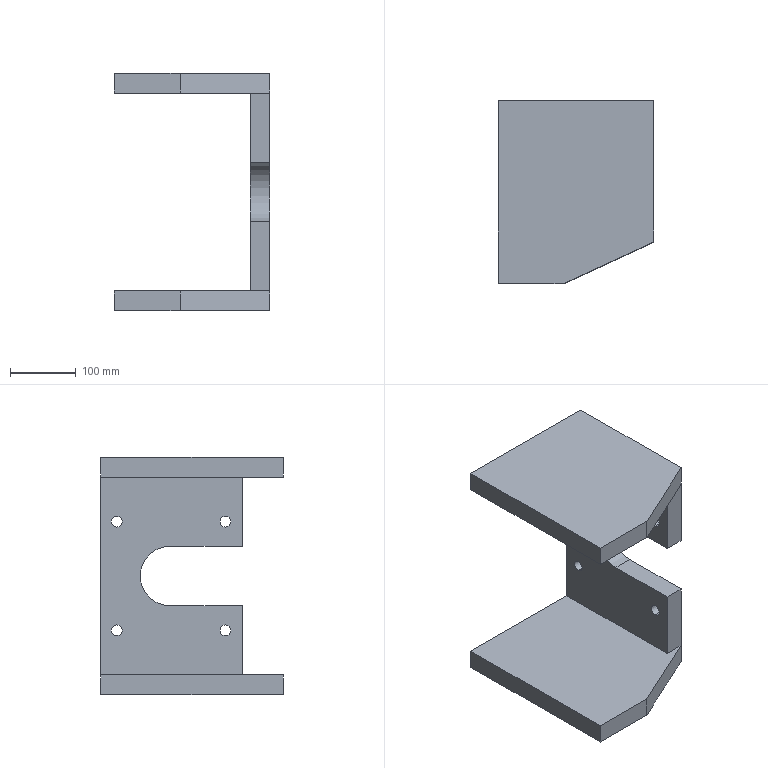Part | SolidWorks | features Extrusion 1, ICE 1, MirrorSolid 1 | 3 solids | 32 faces | box 236 x 277.5 x 360 mm | volume 5191315 mm3 | plane 23 | cylinder 9 | commonest cylinder face diameters 16.5 x8 90 x1
STEP:
#1=CARTESIAN_POINT('',(118.,138.75,0.));
#2=VERTEX_POINT('',#1);
#3=CARTESIAN_POINT('',(-118.,138.75,0.));
#4=VERTEX_POINT('',#3);
#5=CARTESIAN_POINT('',(118.,138.75,0.));
#6=DIRECTION('',(-1.,0.,0.));
#7=VECTOR('',#6,1000.);
#8=LINE('',#5,#7);
#9=EDGE_CURVE('',#2,#4,#8,.T.);
#10=ORIENTED_EDGE('',*,*,#9,.T.);
#11=CARTESIAN_POINT('',(-118.,138.75,30.));
#12=VERTEX_POINT('',#11);
#13=CARTESIAN_POINT('',(-118.,138.75,30.));
#14=DIRECTION('',(0.,0.,-1.));
#15=VECTOR('',#14,1000.);
#16=LINE('',#13,#15);
#17=EDGE_CURVE('',#12,#4,#16,.T.);
#18=ORIENTED_EDGE('',*,*,#17,.F.);
#19=CARTESIAN_POINT('',(118.,138.75,30.));
#20=VERTEX_POINT('',#19);
#21=CARTESIAN_POINT('',(118.,138.75,30.));
#22=DIRECTION('',(-1.,0.,0.));
#23=VECTOR('',#22,1000.);
#24=LINE('',#21,#23);
#25=EDGE_CURVE('',#20,#12,#24,.T.);
#26=ORIENTED_EDGE('',*,*,#25,.F.);
#27=CARTESIAN_POINT('',(118.,138.75,30.));
#28=DIRECTION('',(0.,0.,-1.));
#29=VECTOR('',#28,1000.);
#30=LINE('',#27,#29);
#31=EDGE_CURVE('',#20,#2,#30,.T.);
#32=ORIENTED_EDGE('',*,*,#31,.T.);
#33=EDGE_LOOP('',(#10,#18,#26,#32));
#34=FACE_OUTER_BOUND('',#33,.T.);
#35=CARTESIAN_POINT('',(118.,138.75,30.));
#36=DIRECTION('',(0.,-1.,0.));
#37=DIRECTION('',(1.,0.,0.));
#38=AXIS2_PLACEMENT_3D('',#35,#36,#37);
#39=PLANE('',#38);
#40=ADVANCED_FACE('',(#34),#39,.F.);
#41=CARTESIAN_POINT('',(-118.,-138.75,0.));
#42=VERTEX_POINT('',#41);
#43=CARTESIAN_POINT('',(-118.,138.75,0.));
#44=DIRECTION('',(0.,-1.,0.));
#45=VECTOR('',#44,1000.);
#46=LINE('',#43,#45);
#47=EDGE_CURVE('',#4,#42,#46,.T.);
#48=ORIENTED_EDGE('',*,*,#47,.T.);
#49=CARTESIAN_POINT('',(-118.,-138.75,30.));
#50=VERTEX_POINT('',#49);
#51=CARTESIAN_POINT('',(-118.,-138.75,30.));
#52=DIRECTION('',(0.,0.,-1.));
#53=VECTOR('',#52,1000.);
#54=LINE('',#51,#53);
#55=EDGE_CURVE('',#50,#42,#54,.T.);
#56=ORIENTED_EDGE('',*,*,#55,.F.);
#57=CARTESIAN_POINT('',(-118.,138.75,30.));
#58=DIRECTION('',(0.,-1.,0.));
#59=VECTOR('',#58,1000.);
#60=LINE('',#57,#59);
#61=EDGE_CURVE('',#12,#50,#60,.T.);
#62=ORIENTED_EDGE('',*,*,#61,.F.);
#63=ORIENTED_EDGE('',*,*,#17,.T.);
#64=EDGE_LOOP('',(#48,#56,#62,#63));
#65=FACE_OUTER_BOUND('',#64,.T.);
#66=CARTESIAN_POINT('',(-118.,138.75,30.));
#67=DIRECTION('',(1.,0.,0.));
#68=DIRECTION('',(0.,0.,-1.));
#69=AXIS2_PLACEMENT_3D('',#66,#67,#68);
#70=PLANE('',#69);
#71=ADVANCED_FACE('',(#65),#70,.F.);
#72=CARTESIAN_POINT('',(-18.,-138.75,0.));
#73=VERTEX_POINT('',#72);
#74=CARTESIAN_POINT('',(-18.,-138.75,0.));
#75=DIRECTION('',(1.,0.,0.));
#76=VECTOR('',#75,1000.);
#77=LINE('',#74,#76);
#78=EDGE_CURVE('',#42,#73,#77,.T.);
#79=ORIENTED_EDGE('',*,*,#78,.T.);
#80=CARTESIAN_POINT('',(-18.,-138.75,30.));
#81=VERTEX_POINT('',#80);
#82=CARTESIAN_POINT('',(-18.,-138.75,30.));
#83=DIRECTION('',(0.,0.,-1.));
#84=VECTOR('',#83,1000.);
#85=LINE('',#82,#84);
#86=EDGE_CURVE('',#81,#73,#85,.T.);
#87=ORIENTED_EDGE('',*,*,#86,.F.);
#88=CARTESIAN_POINT('',(-18.,-138.75,30.));
#89=DIRECTION('',(1.,0.,0.));
#90=VECTOR('',#89,1000.);
#91=LINE('',#88,#90);
#92=EDGE_CURVE('',#50,#81,#91,.T.);
#93=ORIENTED_EDGE('',*,*,#92,.F.);
#94=ORIENTED_EDGE('',*,*,#55,.T.);
#95=EDGE_LOOP('',(#79,#87,#93,#94));
#96=FACE_OUTER_BOUND('',#95,.T.);
#97=CARTESIAN_POINT('',(-18.,-138.75,30.));
#98=DIRECTION('',(0.,1.,0.));
#99=DIRECTION('',(-1.,0.,0.));
#100=AXIS2_PLACEMENT_3D('',#97,#98,#99);
#101=PLANE('',#100);
#102=ADVANCED_FACE('',(#96),#101,.F.);
#103=CARTESIAN_POINT('',(118.,-76.25,0.));
#104=VERTEX_POINT('',#103);
#105=CARTESIAN_POINT('',(-18.,-138.75,0.));
#106=DIRECTION('',(0.9086,0.4176,0.));
#107=VECTOR('',#106,1000.);
#108=LINE('',#105,#107);
#109=EDGE_CURVE('',#73,#104,#108,.T.);
#110=ORIENTED_EDGE('',*,*,#109,.T.);
#111=CARTESIAN_POINT('',(118.,-76.25,30.));
#112=VERTEX_POINT('',#111);
#113=CARTESIAN_POINT('',(118.,-76.25,30.));
#114=DIRECTION('',(0.,0.,-1.));
#115=VECTOR('',#114,1000.);
#116=LINE('',#113,#115);
#117=EDGE_CURVE('',#112,#104,#116,.T.);
#118=ORIENTED_EDGE('',*,*,#117,.F.);
#119=CARTESIAN_POINT('',(-18.,-138.75,30.));
#120=DIRECTION('',(0.9086,0.4176,0.));
#121=VECTOR('',#120,1000.);
#122=LINE('',#119,#121);
#123=EDGE_CURVE('',#81,#112,#122,.T.);
#124=ORIENTED_EDGE('',*,*,#123,.F.);
#125=ORIENTED_EDGE('',*,*,#86,.T.);
#126=EDGE_LOOP('',(#110,#118,#124,#125));
#127=FACE_OUTER_BOUND('',#126,.T.);
#128=CARTESIAN_POINT('',(-18.,-138.75,30.));
#129=DIRECTION('',(-0.4176,0.9086,0.));
#130=DIRECTION('',(-0.9086,-0.4176,0.));
#131=AXIS2_PLACEMENT_3D('',#128,#129,#130);
#132=PLANE('',#131);
#133=ADVANCED_FACE('',(#127),#132,.F.);
#134=CARTESIAN_POINT('',(118.,-76.25,0.));
#135=DIRECTION('',(0.,1.,0.));
#136=VECTOR('',#135,1000.);
#137=LINE('',#134,#136);
#138=EDGE_CURVE('',#104,#2,#137,.T.);
#139=ORIENTED_EDGE('',*,*,#138,.T.);
#140=ORIENTED_EDGE('',*,*,#31,.F.);
#141=CARTESIAN_POINT('',(118.,-76.25,30.));
#142=DIRECTION('',(0.,1.,0.));
#143=VECTOR('',#142,1000.);
#144=LINE('',#141,#143);
#145=EDGE_CURVE('',#112,#20,#144,.T.);
#146=ORIENTED_EDGE('',*,*,#145,.F.);
#147=ORIENTED_EDGE('',*,*,#117,.T.);
#148=EDGE_LOOP('',(#139,#140,#146,#147));
#149=FACE_OUTER_BOUND('',#148,.T.);
#150=CARTESIAN_POINT('',(118.,-76.25,30.));
#151=DIRECTION('',(-1.,0.,0.));
#152=DIRECTION('',(0.,0.,1.));
#153=AXIS2_PLACEMENT_3D('',#150,#151,#152);
#154=PLANE('',#153);
#155=ADVANCED_FACE('',(#149),#154,.F.);
#156=ORIENTED_EDGE('',*,*,#25,.T.);
#157=ORIENTED_EDGE('',*,*,#61,.T.);
#158=ORIENTED_EDGE('',*,*,#92,.T.);
#159=ORIENTED_EDGE('',*,*,#123,.T.);
#160=ORIENTED_EDGE('',*,*,#145,.T.);
#161=EDGE_LOOP('',(#156,#157,#158,#159,#160));
#162=FACE_OUTER_BOUND('',#161,.T.);
#163=CARTESIAN_POINT('',(0.,0.,30.));
#164=DIRECTION('',(0.,0.,1.));
#165=DIRECTION('',(1.,0.,0.));
#166=AXIS2_PLACEMENT_3D('',#163,#164,#165);
#167=PLANE('',#166);
#168=ADVANCED_FACE('',(#162),#167,.T.);
#169=ORIENTED_EDGE('',*,*,#9,.F.);
#170=ORIENTED_EDGE('',*,*,#138,.F.);
#171=ORIENTED_EDGE('',*,*,#109,.F.);
#172=ORIENTED_EDGE('',*,*,#78,.F.);
#173=ORIENTED_EDGE('',*,*,#47,.F.);
#174=EDGE_LOOP('',(#169,#170,#171,#172,#173));
#175=FACE_OUTER_BOUND('',#174,.T.);
#176=CARTESIAN_POINT('',(0.,0.,0.));
#177=DIRECTION('',(0.,0.,1.));
#178=DIRECTION('',(1.,0.,0.));
#179=AXIS2_PLACEMENT_3D('',#176,#177,#178);
#180=PLANE('',#179);
#181=ADVANCED_FACE('',(#175),#180,.F.);
#182=CLOSED_SHELL('',(#40,#71,#102,#133,#155,#168,#181));
#183=MANIFOLD_SOLID_BREP('',#182);
#184=CARTESIAN_POINT('',(118.,138.75,-300.));
#185=VERTEX_POINT('',#184);
#186=CARTESIAN_POINT('',(-118.,138.75,-300.));
#187=VERTEX_POINT('',#186);
#188=CARTESIAN_POINT('',(118.,138.75,-300.));
#189=DIRECTION('',(-1.,0.,0.));
#190=VECTOR('',#189,1000.);
#191=LINE('',#188,#190);
#192=EDGE_CURVE('',#185,#187,#191,.T.);
#193=ORIENTED_EDGE('',*,*,#192,.F.);
#194=CARTESIAN_POINT('',(118.,138.75,-330.));
#195=VERTEX_POINT('',#194);
#196=CARTESIAN_POINT('',(118.,138.75,-330.));
#197=DIRECTION('',(0.,0.,1.));
#198=VECTOR('',#197,1000.);
#199=LINE('',#196,#198);
#200=EDGE_CURVE('',#195,#185,#199,.T.);
#201=ORIENTED_EDGE('',*,*,#200,.F.);
#202=CARTESIAN_POINT('',(-118.,138.75,-330.));
#203=VERTEX_POINT('',#202);
#204=CARTESIAN_POINT('',(118.,138.75,-330.));
#205=DIRECTION('',(-1.,0.,0.));
#206=VECTOR('',#205,1000.);
#207=LINE('',#204,#206);
#208=EDGE_CURVE('',#195,#203,#207,.T.);
#209=ORIENTED_EDGE('',*,*,#208,.T.);
#210=CARTESIAN_POINT('',(-118.,138.75,-330.));
#211=DIRECTION('',(0.,0.,1.));
#212=VECTOR('',#211,1000.);
#213=LINE('',#210,#212);
#214=EDGE_CURVE('',#203,#187,#213,.T.);
#215=ORIENTED_EDGE('',*,*,#214,.T.);
#216=EDGE_LOOP('',(#193,#201,#209,#215));
#217=FACE_OUTER_BOUND('',#216,.T.);
#218=CARTESIAN_POINT('',(118.,138.75,-330.));
#219=DIRECTION('',(0.,-1.,0.));
#220=DIRECTION('',(1.,0.,0.));
#221=AXIS2_PLACEMENT_3D('',#218,#219,#220);
#222=PLANE('',#221);
#223=ADVANCED_FACE('',(#217),#222,.F.);
#224=CARTESIAN_POINT('',(-118.,-138.75,-300.));
#225=VERTEX_POINT('',#224);
#226=CARTESIAN_POINT('',(-118.,138.75,-300.));
#227=DIRECTION('',(0.,-1.,0.));
#228=VECTOR('',#227,1000.);
#229=LINE('',#226,#228);
#230=EDGE_CURVE('',#187,#225,#229,.T.);
#231=ORIENTED_EDGE('',*,*,#230,.F.);
#232=ORIENTED_EDGE('',*,*,#214,.F.);
#233=CARTESIAN_POINT('',(-118.,-138.75,-330.));
#234=VERTEX_POINT('',#233);
#235=CARTESIAN_POINT('',(-118.,138.75,-330.));
#236=DIRECTION('',(0.,-1.,0.));
#237=VECTOR('',#236,1000.);
#238=LINE('',#235,#237);
#239=EDGE_CURVE('',#203,#234,#238,.T.);
#240=ORIENTED_EDGE('',*,*,#239,.T.);
#241=CARTESIAN_POINT('',(-118.,-138.75,-330.));
#242=DIRECTION('',(0.,0.,1.));
#243=VECTOR('',#242,1000.);
#244=LINE('',#241,#243);
#245=EDGE_CURVE('',#234,#225,#244,.T.);
#246=ORIENTED_EDGE('',*,*,#245,.T.);
#247=EDGE_LOOP('',(#231,#232,#240,#246));
#248=FACE_OUTER_BOUND('',#247,.T.);
#249=CARTESIAN_POINT('',(-118.,138.75,-330.));
#250=DIRECTION('',(1.,0.,0.));
#251=DIRECTION('',(0.,0.,1.));
#252=AXIS2_PLACEMENT_3D('',#249,#250,#251);
#253=PLANE('',#252);
#254=ADVANCED_FACE('',(#248),#253,.F.);
#255=CARTESIAN_POINT('',(-18.,-138.75,-300.));
#256=VERTEX_POINT('',#255);
#257=CARTESIAN_POINT('',(-18.,-138.75,-300.));
#258=DIRECTION('',(1.,0.,0.));
#259=VECTOR('',#258,1000.);
#260=LINE('',#257,#259);
#261=EDGE_CURVE('',#225,#256,#260,.T.);
#262=ORIENTED_EDGE('',*,*,#261,.F.);
#263=ORIENTED_EDGE('',*,*,#245,.F.);
#264=CARTESIAN_POINT('',(-18.,-138.75,-330.));
#265=VERTEX_POINT('',#264);
#266=CARTESIAN_POINT('',(-18.,-138.75,-330.));
#267=DIRECTION('',(1.,0.,0.));
#268=VECTOR('',#267,1000.);
#269=LINE('',#266,#268);
#270=EDGE_CURVE('',#234,#265,#269,.T.);
#271=ORIENTED_EDGE('',*,*,#270,.T.);
#272=CARTESIAN_POINT('',(-18.,-138.75,-330.));
#273=DIRECTION('',(0.,0.,1.));
#274=VECTOR('',#273,1000.);
#275=LINE('',#272,#274);
#276=EDGE_CURVE('',#265,#256,#275,.T.);
#277=ORIENTED_EDGE('',*,*,#276,.T.);
#278=EDGE_LOOP('',(#262,#263,#271,#277));
#279=FACE_OUTER_BOUND('',#278,.T.);
#280=CARTESIAN_POINT('',(-18.,-138.75,-330.));
#281=DIRECTION('',(0.,1.,0.));
#282=DIRECTION('',(-1.,0.,0.));
#283=AXIS2_PLACEMENT_3D('',#280,#281,#282);
#284=PLANE('',#283);
#285=ADVANCED_FACE('',(#279),#284,.F.);
#286=CARTESIAN_POINT('',(118.,-76.25,-300.));
#287=VERTEX_POINT('',#286);
#288=CARTESIAN_POINT('',(-18.,-138.75,-300.));
#289=DIRECTION('',(0.9086,0.4176,0.));
#290=VECTOR('',#289,1000.);
#291=LINE('',#288,#290);
#292=EDGE_CURVE('',#256,#287,#291,.T.);
#293=ORIENTED_EDGE('',*,*,#292,.F.);
#294=ORIENTED_EDGE('',*,*,#276,.F.);
#295=CARTESIAN_POINT('',(118.,-76.25,-330.));
#296=VERTEX_POINT('',#295);
#297=CARTESIAN_POINT('',(-18.,-138.75,-330.));
#298=DIRECTION('',(0.9086,0.4176,0.));
#299=VECTOR('',#298,1000.);
#300=LINE('',#297,#299);
#301=EDGE_CURVE('',#265,#296,#300,.T.);
#302=ORIENTED_EDGE('',*,*,#301,.T.);
#303=CARTESIAN_POINT('',(118.,-76.25,-330.));
#304=DIRECTION('',(0.,0.,1.));
#305=VECTOR('',#304,1000.);
#306=LINE('',#303,#305);
#307=EDGE_CURVE('',#296,#287,#306,.T.);
#308=ORIENTED_EDGE('',*,*,#307,.T.);
#309=EDGE_LOOP('',(#293,#294,#302,#308));
#310=FACE_OUTER_BOUND('',#309,.T.);
#311=CARTESIAN_POINT('',(-18.,-138.75,-330.));
#312=DIRECTION('',(-0.4176,0.9086,0.));
#313=DIRECTION('',(-0.9086,-0.4176,0.));
#314=AXIS2_PLACEMENT_3D('',#311,#312,#313);
#315=PLANE('',#314);
#316=ADVANCED_FACE('',(#310),#315,.F.);
#317=CARTESIAN_POINT('',(118.,-76.25,-300.));
#318=DIRECTION('',(0.,1.,0.));
#319=VECTOR('',#318,1000.);
#320=LINE('',#317,#319);
#321=EDGE_CURVE('',#287,#185,#320,.T.);
#322=ORIENTED_EDGE('',*,*,#321,.F.);
#323=ORIENTED_EDGE('',*,*,#307,.F.);
#324=CARTESIAN_POINT('',(118.,-76.25,-330.));
#325=DIRECTION('',(0.,1.,0.));
#326=VECTOR('',#325,1000.);
#327=LINE('',#324,#326);
#328=EDGE_CURVE('',#296,#195,#327,.T.);
#329=ORIENTED_EDGE('',*,*,#328,.T.);
#330=ORIENTED_EDGE('',*,*,#200,.T.);
#331=EDGE_LOOP('',(#322,#323,#329,#330));
#332=FACE_OUTER_BOUND('',#331,.T.);
#333=CARTESIAN_POINT('',(118.,-76.25,-330.));
#334=DIRECTION('',(-1.,0.,0.));
#335=DIRECTION('',(0.,0.,-1.));
#336=AXIS2_PLACEMENT_3D('',#333,#334,#335);
#337=PLANE('',#336);
#338=ADVANCED_FACE('',(#332),#337,.F.);
#339=ORIENTED_EDGE('',*,*,#208,.F.);
#340=ORIENTED_EDGE('',*,*,#328,.F.);
#341=ORIENTED_EDGE('',*,*,#301,.F.);
#342=ORIENTED_EDGE('',*,*,#270,.F.);
#343=ORIENTED_EDGE('',*,*,#239,.F.);
#344=EDGE_LOOP('',(#339,#340,#341,#342,#343));
#345=FACE_OUTER_BOUND('',#344,.T.);
#346=CARTESIAN_POINT('',(0.,0.,-330.));
#347=DIRECTION('',(0.,0.,-1.));
#348=DIRECTION('',(1.,0.,0.));
#349=AXIS2_PLACEMENT_3D('',#346,#347,#348);
#350=PLANE('',#349);
#351=ADVANCED_FACE('',(#345),#350,.T.);
#352=ORIENTED_EDGE('',*,*,#192,.T.);
#353=ORIENTED_EDGE('',*,*,#230,.T.);
#354=ORIENTED_EDGE('',*,*,#261,.T.);
#355=ORIENTED_EDGE('',*,*,#292,.T.);
#356=ORIENTED_EDGE('',*,*,#321,.T.);
#357=EDGE_LOOP('',(#352,#353,#354,#355,#356));
#358=FACE_OUTER_BOUND('',#357,.T.);
#359=CARTESIAN_POINT('',(0.,0.,-300.));
#360=DIRECTION('',(0.,0.,-1.));
#361=DIRECTION('',(1.,0.,0.));
#362=AXIS2_PLACEMENT_3D('',#359,#360,#361);
#363=PLANE('',#362);
#364=ADVANCED_FACE('',(#358),#363,.F.);
#365=CLOSED_SHELL('',(#223,#254,#285,#316,#338,#351,#364));
#366=MANIFOLD_SOLID_BREP('',#365);
#367=CARTESIAN_POINT('',(88.,-50.75,-75.75));
#368=VERTEX_POINT('',#367);
#369=CARTESIAN_POINT('',(88.,-50.75,-59.25));
#370=VERTEX_POINT('',#369);
#371=CARTESIAN_POINT('',(88.,-50.75,-67.5));
#372=DIRECTION('',(-1.,0.,0.));
#373=DIRECTION('',(0.,0.,1.));
#374=AXIS2_PLACEMENT_3D('',#371,#372,#373);
#375=CIRCLE('',#374,8.25);
#376=EDGE_CURVE('',#368,#370,#375,.T.);
#377=ORIENTED_EDGE('',*,*,#376,.T.);
#378=CARTESIAN_POINT('',(118.,-50.75,-59.25));
#379=VERTEX_POINT('',#378);
#380=CARTESIAN_POINT('',(88.,-50.75,-59.25));
#381=DIRECTION('',(1.,0.,0.));
#382=VECTOR('',#381,1000.);
#383=LINE('',#380,#382);
#384=EDGE_CURVE('',#370,#379,#383,.T.);
#385=ORIENTED_EDGE('',*,*,#384,.T.);
#386=CARTESIAN_POINT('',(118.,-50.75,-75.75));
#387=VERTEX_POINT('',#386);
#388=CARTESIAN_POINT('',(118.,-50.75,-67.5));
#389=DIRECTION('',(-1.,0.,0.));
#390=DIRECTION('',(0.,0.,1.));
#391=AXIS2_PLACEMENT_3D('',#388,#389,#390);
#392=CIRCLE('',#391,8.25);
#393=EDGE_CURVE('',#387,#379,#392,.T.);
#394=ORIENTED_EDGE('',*,*,#393,.F.);
#395=CARTESIAN_POINT('',(88.,-50.75,-75.75));
#396=DIRECTION('',(1.,0.,0.));
#397=VECTOR('',#396,1000.);
#398=LINE('',#395,#397);
#399=EDGE_CURVE('',#368,#387,#398,.T.);
#400=ORIENTED_EDGE('',*,*,#399,.F.);
#401=EDGE_LOOP('',(#377,#385,#394,#400));
#402=FACE_OUTER_BOUND('',#401,.T.);
#403=CARTESIAN_POINT('',(88.,-50.75,-67.5));
#404=DIRECTION('',(1.,0.,0.));
#405=DIRECTION('',(0.,0.,-1.));
#406=AXIS2_PLACEMENT_3D('',#403,#404,#405);
#407=CYLINDRICAL_SURFACE('',#406,8.25);
#408=ADVANCED_FACE('',(#402),#407,.F.);
#409=CARTESIAN_POINT('',(88.,-50.75,-240.75));
#410=VERTEX_POINT('',#409);
#411=CARTESIAN_POINT('',(88.,-50.75,-224.25));
#412=VERTEX_POINT('',#411);
#413=CARTESIAN_POINT('',(88.,-50.75,-232.5));
#414=DIRECTION('',(-1.,0.,0.));
#415=DIRECTION('',(0.,0.,1.));
#416=AXIS2_PLACEMENT_3D('',#413,#414,#415);
#417=CIRCLE('',#416,8.25);
#418=EDGE_CURVE('',#410,#412,#417,.T.);
#419=ORIENTED_EDGE('',*,*,#418,.T.);
#420=CARTESIAN_POINT('',(118.,-50.75,-224.25));
#421=VERTEX_POINT('',#420);
#422=CARTESIAN_POINT('',(88.,-50.75,-224.25));
#423=DIRECTION('',(1.,0.,0.));
#424=VECTOR('',#423,1000.);
#425=LINE('',#422,#424);
#426=EDGE_CURVE('',#412,#421,#425,.T.);
#427=ORIENTED_EDGE('',*,*,#426,.T.);
#428=CARTESIAN_POINT('',(118.,-50.75,-240.75));
#429=VERTEX_POINT('',#428);
#430=CARTESIAN_POINT('',(118.,-50.75,-232.5));
#431=DIRECTION('',(-1.,0.,0.));
#432=DIRECTION('',(0.,0.,1.));
#433=AXIS2_PLACEMENT_3D('',#430,#431,#432);
#434=CIRCLE('',#433,8.25);
#435=EDGE_CURVE('',#429,#421,#434,.T.);
#436=ORIENTED_EDGE('',*,*,#435,.F.);
#437=CARTESIAN_POINT('',(88.,-50.75,-240.75));
#438=DIRECTION('',(1.,0.,0.));
#439=VECTOR('',#438,1000.);
#440=LINE('',#437,#439);
#441=EDGE_CURVE('',#410,#429,#440,.T.);
#442=ORIENTED_EDGE('',*,*,#441,.F.);
#443=EDGE_LOOP('',(#419,#427,#436,#442));
#444=FACE_OUTER_BOUND('',#443,.T.);
#445=CARTESIAN_POINT('',(88.,-50.75,-232.5));
#446=DIRECTION('',(1.,0.,0.));
#447=DIRECTION('',(0.,0.,-1.));
#448=AXIS2_PLACEMENT_3D('',#445,#446,#447);
#449=CYLINDRICAL_SURFACE('',#448,8.25);
#450=ADVANCED_FACE('',(#444),#449,.F.);
#451=CARTESIAN_POINT('',(88.,114.25,-240.75));
#452=VERTEX_POINT('',#451);
#453=CARTESIAN_POINT('',(88.,114.25,-224.25));
#454=VERTEX_POINT('',#453);
#455=CARTESIAN_POINT('',(88.,114.25,-232.5));
#456=DIRECTION('',(-1.,0.,0.));
#457=DIRECTION('',(0.,0.,1.));
#458=AXIS2_PLACEMENT_3D('',#455,#456,#457);
#459=CIRCLE('',#458,8.25);
#460=EDGE_CURVE('',#452,#454,#459,.T.);
#461=ORIENTED_EDGE('',*,*,#460,.T.);
#462=CARTESIAN_POINT('',(118.,114.25,-224.25));
#463=VERTEX_POINT('',#462);
#464=CARTESIAN_POINT('',(88.,114.25,-224.25));
#465=DIRECTION('',(1.,0.,0.));
#466=VECTOR('',#465,1000.);
#467=LINE('',#464,#466);
#468=EDGE_CURVE('',#454,#463,#467,.T.);
#469=ORIENTED_EDGE('',*,*,#468,.T.);
#470=CARTESIAN_POINT('',(118.,114.25,-240.75));
#471=VERTEX_POINT('',#470);
#472=CARTESIAN_POINT('',(118.,114.25,-232.5));
#473=DIRECTION('',(-1.,0.,0.));
#474=DIRECTION('',(0.,0.,1.));
#475=AXIS2_PLACEMENT_3D('',#472,#473,#474);
#476=CIRCLE('',#475,8.25);
#477=EDGE_CURVE('',#471,#463,#476,.T.);
#478=ORIENTED_EDGE('',*,*,#477,.F.);
#479=CARTESIAN_POINT('',(88.,114.25,-240.75));
#480=DIRECTION('',(1.,0.,0.));
#481=VECTOR('',#480,1000.);
#482=LINE('',#479,#481);
#483=EDGE_CURVE('',#452,#471,#482,.T.);
#484=ORIENTED_EDGE('',*,*,#483,.F.);
#485=EDGE_LOOP('',(#461,#469,#478,#484));
#486=FACE_OUTER_BOUND('',#485,.T.);
#487=CARTESIAN_POINT('',(88.,114.25,-232.5));
#488=DIRECTION('',(1.,0.,0.));
#489=DIRECTION('',(0.,0.,-1.));
#490=AXIS2_PLACEMENT_3D('',#487,#488,#489);
#491=CYLINDRICAL_SURFACE('',#490,8.25);
#492=ADVANCED_FACE('',(#486),#491,.F.);
#493=CARTESIAN_POINT('',(88.,114.25,-75.75));
#494=VERTEX_POINT('',#493);
#495=CARTESIAN_POINT('',(88.,114.25,-59.25));
#496=VERTEX_POINT('',#495);
#497=CARTESIAN_POINT('',(88.,114.25,-67.5));
#498=DIRECTION('',(-1.,0.,0.));
#499=DIRECTION('',(0.,0.,1.));
#500=AXIS2_PLACEMENT_3D('',#497,#498,#499);
#501=CIRCLE('',#500,8.25);
#502=EDGE_CURVE('',#494,#496,#501,.T.);
#503=ORIENTED_EDGE('',*,*,#502,.T.);
#504=CARTESIAN_POINT('',(118.,114.25,-59.25));
#505=VERTEX_POINT('',#504);
#506=CARTESIAN_POINT('',(88.,114.25,-59.25));
#507=DIRECTION('',(1.,0.,0.));
#508=VECTOR('',#507,1000.);
#509=LINE('',#506,#508);
#510=EDGE_CURVE('',#496,#505,#509,.T.);
#511=ORIENTED_EDGE('',*,*,#510,.T.);
#512=CARTESIAN_POINT('',(118.,114.25,-75.75));
#513=VERTEX_POINT('',#512);
#514=CARTESIAN_POINT('',(118.,114.25,-67.5));
#515=DIRECTION('',(-1.,0.,0.));
#516=DIRECTION('',(0.,0.,1.));
#517=AXIS2_PLACEMENT_3D('',#514,#515,#516);
#518=CIRCLE('',#517,8.25);
#519=EDGE_CURVE('',#513,#505,#518,.T.);
#520=ORIENTED_EDGE('',*,*,#519,.F.);
#521=CARTESIAN_POINT('',(88.,114.25,-75.75));
#522=DIRECTION('',(1.,0.,0.));
#523=VECTOR('',#522,1000.);
#524=LINE('',#521,#523);
#525=EDGE_CURVE('',#494,#513,#524,.T.);
#526=ORIENTED_EDGE('',*,*,#525,.F.);
#527=EDGE_LOOP('',(#503,#511,#520,#526));
#528=FACE_OUTER_BOUND('',#527,.T.);
#529=CARTESIAN_POINT('',(88.,114.25,-67.5));
#530=DIRECTION('',(1.,0.,0.));
#531=DIRECTION('',(0.,0.,-1.));
#532=AXIS2_PLACEMENT_3D('',#529,#530,#531);
#533=CYLINDRICAL_SURFACE('',#532,8.25);
#534=ADVANCED_FACE('',(#528),#533,.F.);
#535=ORIENTED_EDGE('',*,*,#418,.F.);
#536=CARTESIAN_POINT('',(88.,-50.75,-232.5));
#537=DIRECTION('',(-1.,0.,0.));
#538=DIRECTION('',(0.,0.,1.));
#539=AXIS2_PLACEMENT_3D('',#536,#537,#538);
#540=CIRCLE('',#539,8.25);
#541=EDGE_CURVE('',#412,#410,#540,.T.);
#542=ORIENTED_EDGE('',*,*,#541,.F.);
#543=EDGE_LOOP('',(#535,#542));
#544=FACE_BOUND('',#543,.T.);
#545=ORIENTED_EDGE('',*,*,#502,.F.);
#546=CARTESIAN_POINT('',(88.,114.25,-67.5));
#547=DIRECTION('',(-1.,0.,0.));
#548=DIRECTION('',(0.,0.,1.));
#549=AXIS2_PLACEMENT_3D('',#546,#547,#548);
#550=CIRCLE('',#549,8.25);
#551=EDGE_CURVE('',#496,#494,#550,.T.);
#552=ORIENTED_EDGE('',*,*,#551,.F.);
#553=EDGE_LOOP('',(#545,#552));
#554=FACE_BOUND('',#553,.T.);
#555=CARTESIAN_POINT('',(88.,-76.25,-300.));
#556=VERTEX_POINT('',#555);
#557=CARTESIAN_POINT('',(88.,138.75,-300.));
#558=VERTEX_POINT('',#557);
#559=CARTESIAN_POINT('',(88.,-76.25,-300.));
#560=DIRECTION('',(0.,1.,0.));
#561=VECTOR('',#560,1000.);
#562=LINE('',#559,#561);
#563=EDGE_CURVE('',#556,#558,#562,.T.);
#564=ORIENTED_EDGE('',*,*,#563,.F.);
#565=CARTESIAN_POINT('',(88.,-76.25,-195.));
#566=VERTEX_POINT('',#565);
#567=CARTESIAN_POINT('',(88.,-76.25,30.));
#568=DIRECTION('',(0.,0.,-1.));
#569=VECTOR('',#568,1000.);
#570=LINE('',#567,#569);
#571=EDGE_CURVE('',#566,#556,#570,.T.);
#572=ORIENTED_EDGE('',*,*,#571,.F.);
#573=CARTESIAN_POINT('',(88.,33.75,-195.));
#574=VERTEX_POINT('',#573);
#575=CARTESIAN_POINT('',(88.,-76.25,-195.));
#576=DIRECTION('',(0.,-1.,0.));
#577=VECTOR('',#576,1000.);
#578=LINE('',#575,#577);
#579=EDGE_CURVE('',#574,#566,#578,.T.);
#580=ORIENTED_EDGE('',*,*,#579,.F.);
#581=CARTESIAN_POINT('',(88.,33.75,-105.));
#582=VERTEX_POINT('',#581);
#583=CARTESIAN_POINT('',(88.,33.75,-150.));
#584=DIRECTION('',(-1.,0.,0.));
#585=DIRECTION('',(0.,0.,1.));
#586=AXIS2_PLACEMENT_3D('',#583,#584,#585);
#587=CIRCLE('',#586,45.);
#588=EDGE_CURVE('',#582,#574,#587,.T.);
#589=ORIENTED_EDGE('',*,*,#588,.F.);
#590=CARTESIAN_POINT('',(88.,-76.25,-105.));
#591=VERTEX_POINT('',#590);
#592=CARTESIAN_POINT('',(88.,-76.25,-105.));
#593=DIRECTION('',(0.,1.,0.));
#594=VECTOR('',#593,1000.);
#595=LINE('',#592,#594);
#596=EDGE_CURVE('',#591,#582,#595,.T.);
#597=ORIENTED_EDGE('',*,*,#596,.F.);
#598=CARTESIAN_POINT('',(88.,-76.25,0.));
#599=VERTEX_POINT('',#598);
#600=CARTESIAN_POINT('',(88.,-76.25,30.));
#601=DIRECTION('',(0.,0.,-1.));
#602=VECTOR('',#601,1000.);
#603=LINE('',#600,#602);
#604=EDGE_CURVE('',#599,#591,#603,.T.);
#605=ORIENTED_EDGE('',*,*,#604,.F.);
#606=CARTESIAN_POINT('',(88.,138.75,0.));
#607=VERTEX_POINT('',#606);
#608=CARTESIAN_POINT('',(88.,-76.25,0.));
#609=DIRECTION('',(0.,-1.,0.));
#610=VECTOR('',#609,1000.);
#611=LINE('',#608,#610);
#612=EDGE_CURVE('',#607,#599,#611,.T.);
#613=ORIENTED_EDGE('',*,*,#612,.F.);
#614=CARTESIAN_POINT('',(88.,138.75,30.));
#615=DIRECTION('',(0.,0.,1.));
#616=VECTOR('',#615,1000.);
#617=LINE('',#614,#616);
#618=EDGE_CURVE('',#558,#607,#617,.T.);
#619=ORIENTED_EDGE('',*,*,#618,.F.);
#620=EDGE_LOOP('',(#564,#572,#580,#589,#597,#605,#613,#619));
#621=FACE_OUTER_BOUND('',#620,.T.);
#622=ORIENTED_EDGE('',*,*,#460,.F.);
#623=CARTESIAN_POINT('',(88.,114.25,-232.5));
#624=DIRECTION('',(-1.,0.,0.));
#625=DIRECTION('',(0.,0.,1.));
#626=AXIS2_PLACEMENT_3D('',#623,#624,#625);
#627=CIRCLE('',#626,8.25);
#628=EDGE_CURVE('',#454,#452,#627,.T.);
#629=ORIENTED_EDGE('',*,*,#628,.F.);
#630=EDGE_LOOP('',(#622,#629));
#631=FACE_BOUND('',#630,.T.);
#632=ORIENTED_EDGE('',*,*,#376,.F.);
#633=CARTESIAN_POINT('',(88.,-50.75,-67.5));
#634=DIRECTION('',(-1.,0.,0.));
#635=DIRECTION('',(0.,0.,1.));
#636=AXIS2_PLACEMENT_3D('',#633,#634,#635);
#637=CIRCLE('',#636,8.25);
#638=EDGE_CURVE('',#370,#368,#637,.T.);
#639=ORIENTED_EDGE('',*,*,#638,.F.);
#640=EDGE_LOOP('',(#632,#639));
#641=FACE_BOUND('',#640,.T.);
#642=CARTESIAN_POINT('',(88.,33.75,-150.));
#643=DIRECTION('',(-1.,0.,0.));
#644=DIRECTION('',(0.,0.,1.));
#645=AXIS2_PLACEMENT_3D('',#642,#643,#644);
#646=PLANE('',#645);
#647=ADVANCED_FACE('',(#544,#554,#621,#631,#641),#646,.T.);
#648=CARTESIAN_POINT('',(118.,-76.25,-300.));
#649=VERTEX_POINT('',#648);
#650=CARTESIAN_POINT('',(118.,138.75,-300.));
#651=VERTEX_POINT('',#650);
#652=CARTESIAN_POINT('',(118.,-76.25,-300.));
#653=DIRECTION('',(0.,1.,0.));
#654=VECTOR('',#653,1000.);
#655=LINE('',#652,#654);
#656=EDGE_CURVE('',#649,#651,#655,.T.);
#657=ORIENTED_EDGE('',*,*,#656,.T.);
#658=CARTESIAN_POINT('',(118.,138.75,0.));
#659=VERTEX_POINT('',#658);
#660=CARTESIAN_POINT('',(118.,138.75,30.));
#661=DIRECTION('',(0.,0.,1.));
#662=VECTOR('',#661,1000.);
#663=LINE('',#660,#662);
#664=EDGE_CURVE('',#651,#659,#663,.T.);
#665=ORIENTED_EDGE('',*,*,#664,.T.);
#666=CARTESIAN_POINT('',(118.,-76.25,0.));
#667=VERTEX_POINT('',#666);
#668=CARTESIAN_POINT('',(118.,-76.25,0.));
#669=DIRECTION('',(0.,-1.,0.));
#670=VECTOR('',#669,1000.);
#671=LINE('',#668,#670);
#672=EDGE_CURVE('',#659,#667,#671,.T.);
#673=ORIENTED_EDGE('',*,*,#672,.T.);
#674=CARTESIAN_POINT('',(118.,-76.25,-105.));
#675=VERTEX_POINT('',#674);
#676=CARTESIAN_POINT('',(118.,-76.25,30.));
#677=DIRECTION('',(0.,0.,-1.));
#678=VECTOR('',#677,1000.);
#679=LINE('',#676,#678);
#680=EDGE_CURVE('',#667,#675,#679,.T.);
#681=ORIENTED_EDGE('',*,*,#680,.T.);
#682=CARTESIAN_POINT('',(118.,33.75,-105.));
#683=VERTEX_POINT('',#682);
#684=CARTESIAN_POINT('',(118.,-76.25,-105.));
#685=DIRECTION('',(0.,1.,0.));
#686=VECTOR('',#685,1000.);
#687=LINE('',#684,#686);
#688=EDGE_CURVE('',#675,#683,#687,.T.);
#689=ORIENTED_EDGE('',*,*,#688,.T.);
#690=CARTESIAN_POINT('',(118.,33.75,-195.));
#691=VERTEX_POINT('',#690);
#692=CARTESIAN_POINT('',(118.,33.75,-150.));
#693=DIRECTION('',(-1.,0.,0.));
#694=DIRECTION('',(0.,0.,1.));
#695=AXIS2_PLACEMENT_3D('',#692,#693,#694);
#696=CIRCLE('',#695,45.);
#697=EDGE_CURVE('',#683,#691,#696,.T.);
#698=ORIENTED_EDGE('',*,*,#697,.T.);
#699=CARTESIAN_POINT('',(118.,-76.25,-195.));
#700=VERTEX_POINT('',#699);
#701=CARTESIAN_POINT('',(118.,-76.25,-195.));
#702=DIRECTION('',(0.,-1.,0.));
#703=VECTOR('',#702,1000.);
#704=LINE('',#701,#703);
#705=EDGE_CURVE('',#691,#700,#704,.T.);
#706=ORIENTED_EDGE('',*,*,#705,.T.);
#707=CARTESIAN_POINT('',(118.,-76.25,30.));
#708=DIRECTION('',(0.,0.,-1.));
#709=VECTOR('',#708,1000.);
#710=LINE('',#707,#709);
#711=EDGE_CURVE('',#700,#649,#710,.T.);
#712=ORIENTED_EDGE('',*,*,#711,.T.);
#713=EDGE_LOOP('',(#657,#665,#673,#681,#689,#698,#706,#712));
#714=FACE_OUTER_BOUND('',#713,.T.);
#715=ORIENTED_EDGE('',*,*,#519,.T.);
#716=CARTESIAN_POINT('',(118.,114.25,-67.5));
#717=DIRECTION('',(-1.,0.,0.));
#718=DIRECTION('',(0.,0.,1.));
#719=AXIS2_PLACEMENT_3D('',#716,#717,#718);
#720=CIRCLE('',#719,8.25);
#721=EDGE_CURVE('',#505,#513,#720,.T.);
#722=ORIENTED_EDGE('',*,*,#721,.T.);
#723=EDGE_LOOP('',(#715,#722));
#724=FACE_BOUND('',#723,.T.);
#725=ORIENTED_EDGE('',*,*,#477,.T.);
#726=CARTESIAN_POINT('',(118.,114.25,-232.5));
#727=DIRECTION('',(-1.,0.,0.));
#728=DIRECTION('',(0.,0.,1.));
#729=AXIS2_PLACEMENT_3D('',#726,#727,#728);
#730=CIRCLE('',#729,8.25);
#731=EDGE_CURVE('',#463,#471,#730,.T.);
#732=ORIENTED_EDGE('',*,*,#731,.T.);
#733=EDGE_LOOP('',(#725,#732));
#734=FACE_BOUND('',#733,.T.);
#735=ORIENTED_EDGE('',*,*,#435,.T.);
#736=CARTESIAN_POINT('',(118.,-50.75,-232.5));
#737=DIRECTION('',(-1.,0.,0.));
#738=DIRECTION('',(0.,0.,1.));
#739=AXIS2_PLACEMENT_3D('',#736,#737,#738);
#740=CIRCLE('',#739,8.25);
#741=EDGE_CURVE('',#421,#429,#740,.T.);
#742=ORIENTED_EDGE('',*,*,#741,.T.);
#743=EDGE_LOOP('',(#735,#742));
#744=FACE_BOUND('',#743,.T.);
#745=ORIENTED_EDGE('',*,*,#393,.T.);
#746=CARTESIAN_POINT('',(118.,-50.75,-67.5));
#747=DIRECTION('',(-1.,0.,0.));
#748=DIRECTION('',(0.,0.,1.));
#749=AXIS2_PLACEMENT_3D('',#746,#747,#748);
#750=CIRCLE('',#749,8.25);
#751=EDGE_CURVE('',#379,#387,#750,.T.);
#752=ORIENTED_EDGE('',*,*,#751,.T.);
#753=EDGE_LOOP('',(#745,#752));
#754=FACE_BOUND('',#753,.T.);
#755=CARTESIAN_POINT('',(118.,33.75,-150.));
#756=DIRECTION('',(-1.,0.,0.));
#757=DIRECTION('',(0.,0.,1.));
#758=AXIS2_PLACEMENT_3D('',#755,#756,#757);
#759=PLANE('',#758);
#760=ADVANCED_FACE('',(#714,#724,#734,#744,#754),#759,.F.);
#761=ORIENTED_EDGE('',*,*,#656,.F.);
#762=CARTESIAN_POINT('',(88.,-76.25,-300.));
#763=DIRECTION('',(1.,0.,0.));
#764=VECTOR('',#763,1000.);
#765=LINE('',#762,#764);
#766=EDGE_CURVE('',#556,#649,#765,.T.);
#767=ORIENTED_EDGE('',*,*,#766,.F.);
#768=ORIENTED_EDGE('',*,*,#563,.T.);
#769=CARTESIAN_POINT('',(88.,138.75,-300.));
#770=DIRECTION('',(1.,0.,0.));
#771=VECTOR('',#770,1000.);
#772=LINE('',#769,#771);
#773=EDGE_CURVE('',#558,#651,#772,.T.);
#774=ORIENTED_EDGE('',*,*,#773,.T.);
#775=EDGE_LOOP('',(#761,#767,#768,#774));
#776=FACE_OUTER_BOUND('',#775,.T.);
#777=CARTESIAN_POINT('',(88.,-76.25,-300.));
#778=DIRECTION('',(0.,0.,-1.));
#779=DIRECTION('',(-1.,0.,0.));
#780=AXIS2_PLACEMENT_3D('',#777,#778,#779);
#781=PLANE('',#780);
#782=ADVANCED_FACE('',(#776),#781,.T.);
#783=ORIENTED_EDGE('',*,*,#711,.F.);
#784=CARTESIAN_POINT('',(88.,-76.25,-195.));
#785=DIRECTION('',(1.,0.,0.));
#786=VECTOR('',#785,1000.);
#787=LINE('',#784,#786);
#788=EDGE_CURVE('',#566,#700,#787,.T.);
#789=ORIENTED_EDGE('',*,*,#788,.F.);
#790=ORIENTED_EDGE('',*,*,#571,.T.);
#791=ORIENTED_EDGE('',*,*,#766,.T.);
#792=EDGE_LOOP('',(#783,#789,#790,#791));
#793=FACE_OUTER_BOUND('',#792,.T.);
#794=CARTESIAN_POINT('',(88.,-76.25,30.));
#795=DIRECTION('',(0.,-1.,0.));
#796=DIRECTION('',(0.,0.,-1.));
#797=AXIS2_PLACEMENT_3D('',#794,#795,#796);
#798=PLANE('',#797);
#799=ADVANCED_FACE('',(#793),#798,.T.);
#800=ORIENTED_EDGE('',*,*,#705,.F.);
#801=CARTESIAN_POINT('',(88.,33.75,-195.));
#802=DIRECTION('',(1.,0.,0.));
#803=VECTOR('',#802,1000.);
#804=LINE('',#801,#803);
#805=EDGE_CURVE('',#574,#691,#804,.T.);
#806=ORIENTED_EDGE('',*,*,#805,.F.);
#807=ORIENTED_EDGE('',*,*,#579,.T.);
#808=ORIENTED_EDGE('',*,*,#788,.T.);
#809=EDGE_LOOP('',(#800,#806,#807,#808));
#810=FACE_OUTER_BOUND('',#809,.T.);
#811=CARTESIAN_POINT('',(88.,-76.25,-195.));
#812=DIRECTION('',(0.,0.,1.));
#813=DIRECTION('',(1.,0.,0.));
#814=AXIS2_PLACEMENT_3D('',#811,#812,#813);
#815=PLANE('',#814);
#816=ADVANCED_FACE('',(#810),#815,.T.);
#817=ORIENTED_EDGE('',*,*,#697,.F.);
#818=CARTESIAN_POINT('',(88.,33.75,-105.));
#819=DIRECTION('',(1.,0.,0.));
#820=VECTOR('',#819,1000.);
#821=LINE('',#818,#820);
#822=EDGE_CURVE('',#582,#683,#821,.T.);
#823=ORIENTED_EDGE('',*,*,#822,.F.);
#824=ORIENTED_EDGE('',*,*,#588,.T.);
#825=ORIENTED_EDGE('',*,*,#805,.T.);
#826=EDGE_LOOP('',(#817,#823,#824,#825));
#827=FACE_OUTER_BOUND('',#826,.T.);
#828=CARTESIAN_POINT('',(88.,33.75,-150.));
#829=DIRECTION('',(1.,0.,0.));
#830=DIRECTION('',(0.,0.,-1.));
#831=AXIS2_PLACEMENT_3D('',#828,#829,#830);
#832=CYLINDRICAL_SURFACE('',#831,45.);
#833=ADVANCED_FACE('',(#827),#832,.F.);
#834=ORIENTED_EDGE('',*,*,#688,.F.);
#835=CARTESIAN_POINT('',(88.,-76.25,-105.));
#836=DIRECTION('',(1.,0.,0.));
#837=VECTOR('',#836,1000.);
#838=LINE('',#835,#837);
#839=EDGE_CURVE('',#591,#675,#838,.T.);
#840=ORIENTED_EDGE('',*,*,#839,.F.);
#841=ORIENTED_EDGE('',*,*,#596,.T.);
#842=ORIENTED_EDGE('',*,*,#822,.T.);
#843=EDGE_LOOP('',(#834,#840,#841,#842));
#844=FACE_OUTER_BOUND('',#843,.T.);
#845=CARTESIAN_POINT('',(88.,-76.25,-105.));
#846=DIRECTION('',(0.,0.,-1.));
#847=DIRECTION('',(0.,1.,0.));
#848=AXIS2_PLACEMENT_3D('',#845,#846,#847);
#849=PLANE('',#848);
#850=ADVANCED_FACE('',(#844),#849,.T.);
#851=ORIENTED_EDGE('',*,*,#680,.F.);
#852=CARTESIAN_POINT('',(88.,-76.25,0.));
#853=DIRECTION('',(1.,0.,0.));
#854=VECTOR('',#853,1000.);
#855=LINE('',#852,#854);
#856=EDGE_CURVE('',#599,#667,#855,.T.);
#857=ORIENTED_EDGE('',*,*,#856,.F.);
#858=ORIENTED_EDGE('',*,*,#604,.T.);
#859=ORIENTED_EDGE('',*,*,#839,.T.);
#860=EDGE_LOOP('',(#851,#857,#858,#859));
#861=FACE_OUTER_BOUND('',#860,.T.);
#862=CARTESIAN_POINT('',(88.,-76.25,30.));
#863=DIRECTION('',(0.,-1.,0.));
#864=DIRECTION('',(0.,0.,-1.));
#865=AXIS2_PLACEMENT_3D('',#862,#863,#864);
#866=PLANE('',#865);
#867=ADVANCED_FACE('',(#861),#866,.T.);
#868=ORIENTED_EDGE('',*,*,#672,.F.);
#869=CARTESIAN_POINT('',(88.,138.75,0.));
#870=DIRECTION('',(1.,0.,0.));
#871=VECTOR('',#870,1000.);
#872=LINE('',#869,#871);
#873=EDGE_CURVE('',#607,#659,#872,.T.);
#874=ORIENTED_EDGE('',*,*,#873,.F.);
#875=ORIENTED_EDGE('',*,*,#612,.T.);
#876=ORIENTED_EDGE('',*,*,#856,.T.);
#877=EDGE_LOOP('',(#868,#874,#875,#876));
#878=FACE_OUTER_BOUND('',#877,.T.);
#879=CARTESIAN_POINT('',(88.,-76.25,0.));
#880=DIRECTION('',(0.,0.,1.));
#881=DIRECTION('',(0.,-1.,0.));
#882=AXIS2_PLACEMENT_3D('',#879,#880,#881);
#883=PLANE('',#882);
#884=ADVANCED_FACE('',(#878),#883,.T.);
#885=ORIENTED_EDGE('',*,*,#664,.F.);
#886=ORIENTED_EDGE('',*,*,#773,.F.);
#887=ORIENTED_EDGE('',*,*,#618,.T.);
#888=ORIENTED_EDGE('',*,*,#873,.T.);
#889=EDGE_LOOP('',(#885,#886,#887,#888));
#890=FACE_OUTER_BOUND('',#889,.T.);
#891=CARTESIAN_POINT('',(88.,138.75,30.));
#892=DIRECTION('',(0.,1.,0.));
#893=DIRECTION('',(0.,0.,1.));
#894=AXIS2_PLACEMENT_3D('',#891,#892,#893);
#895=PLANE('',#894);
#896=ADVANCED_FACE('',(#890),#895,.T.);
#897=ORIENTED_EDGE('',*,*,#510,.F.);
#898=ORIENTED_EDGE('',*,*,#551,.T.);
#899=ORIENTED_EDGE('',*,*,#525,.T.);
#900=ORIENTED_EDGE('',*,*,#721,.F.);
#901=EDGE_LOOP('',(#897,#898,#899,#900));
#902=FACE_OUTER_BOUND('',#901,.T.);
#903=CARTESIAN_POINT('',(88.,114.25,-67.5));
#904=DIRECTION('',(1.,0.,0.));
#905=DIRECTION('',(0.,0.,-1.));
#906=AXIS2_PLACEMENT_3D('',#903,#904,#905);
#907=CYLINDRICAL_SURFACE('',#906,8.25);
#908=ADVANCED_FACE('',(#902),#907,.F.);
#909=ORIENTED_EDGE('',*,*,#468,.F.);
#910=ORIENTED_EDGE('',*,*,#628,.T.);
#911=ORIENTED_EDGE('',*,*,#483,.T.);
#912=ORIENTED_EDGE('',*,*,#731,.F.);
#913=EDGE_LOOP('',(#909,#910,#911,#912));
#914=FACE_OUTER_BOUND('',#913,.T.);
#915=CARTESIAN_POINT('',(88.,114.25,-232.5));
#916=DIRECTION('',(1.,0.,0.));
#917=DIRECTION('',(0.,0.,-1.));
#918=AXIS2_PLACEMENT_3D('',#915,#916,#917);
#919=CYLINDRICAL_SURFACE('',#918,8.25);
#920=ADVANCED_FACE('',(#914),#919,.F.);
#921=ORIENTED_EDGE('',*,*,#426,.F.);
#922=ORIENTED_EDGE('',*,*,#541,.T.);
#923=ORIENTED_EDGE('',*,*,#441,.T.);
#924=ORIENTED_EDGE('',*,*,#741,.F.);
#925=EDGE_LOOP('',(#921,#922,#923,#924));
#926=FACE_OUTER_BOUND('',#925,.T.);
#927=CARTESIAN_POINT('',(88.,-50.75,-232.5));
#928=DIRECTION('',(1.,0.,0.));
#929=DIRECTION('',(0.,0.,-1.));
#930=AXIS2_PLACEMENT_3D('',#927,#928,#929);
#931=CYLINDRICAL_SURFACE('',#930,8.25);
#932=ADVANCED_FACE('',(#926),#931,.F.);
#933=ORIENTED_EDGE('',*,*,#384,.F.);
#934=ORIENTED_EDGE('',*,*,#638,.T.);
#935=ORIENTED_EDGE('',*,*,#399,.T.);
#936=ORIENTED_EDGE('',*,*,#751,.F.);
#937=EDGE_LOOP('',(#933,#934,#935,#936));
#938=FACE_OUTER_BOUND('',#937,.T.);
#939=CARTESIAN_POINT('',(88.,-50.75,-67.5));
#940=DIRECTION('',(1.,0.,0.));
#941=DIRECTION('',(0.,0.,-1.));
#942=AXIS2_PLACEMENT_3D('',#939,#940,#941);
#943=CYLINDRICAL_SURFACE('',#942,8.25);
#944=ADVANCED_FACE('',(#938),#943,.F.);
#945=CLOSED_SHELL('',(#408,#450,#492,#534,#647,#760,#782,#799,#816,#833,#850,#867,#884,#896,#908,#920,#932,#944));
#946=MANIFOLD_SOLID_BREP('',#945);
#947=CARTESIAN_POINT('',(0.,0.,0.));
#948=DIRECTION('',(0.,0.,1.));
#949=DIRECTION('',(1.,0.,0.));
#950=AXIS2_PLACEMENT_3D('',#947,#948,#949);
#951=(LENGTH_UNIT()NAMED_UNIT(*)SI_UNIT(.MILLI.,.METRE.));
#952=UNCERTAINTY_MEASURE_WITH_UNIT(LENGTH_MEASURE(0.00001),#951,'','');
#953=(NAMED_UNIT(*)PLANE_ANGLE_UNIT()SI_UNIT($,.RADIAN.));
#954=(NAMED_UNIT(*)SI_UNIT($,.STERADIAN.)SOLID_ANGLE_UNIT());
#955=(GEOMETRIC_REPRESENTATION_CONTEXT(3)GLOBAL_UNCERTAINTY_ASSIGNED_CONTEXT((#952))GLOBAL_UNIT_ASSIGNED_CONTEXT((#951,#953,#954))REPRESENTATION_CONTEXT('',''));
#956=ADVANCED_BREP_SHAPE_REPRESENTATION('',(#183,#366,#946,#950),#955);